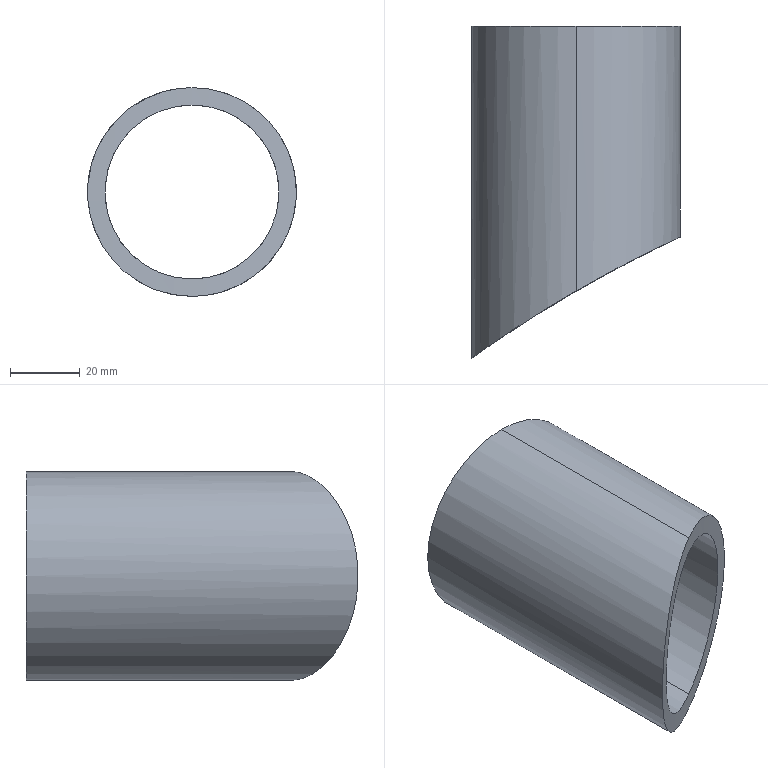Part | SolidWorks | features Extrusion 1, ICE 1 | 1 solid | 6 faces | box 60 x 95.435 x 60 mm | volume 66487 mm3 | cylinder 5 | plane 1 | commonest cylinder face diameters 50 x2 60 x2 759 x1
STEP:
#1=CARTESIAN_POINT('',(0.,300.,-25.));
#2=VERTEX_POINT('',#1);
#3=CARTESIAN_POINT('',(0.,300.,25.));
#4=VERTEX_POINT('',#3);
#5=CARTESIAN_POINT('',(0.,300.,0.));
#6=DIRECTION('',(0.,1.,0.));
#7=DIRECTION('',(0.,0.,1.));
#8=AXIS2_PLACEMENT_3D('',#5,#6,#7);
#9=CIRCLE('',#8,25.);
#10=EDGE_CURVE('',#2,#4,#9,.T.);
#11=ORIENTED_EDGE('',*,*,#10,.T.);
#12=CARTESIAN_POINT('',(0.,223.819,25.));
#13=VERTEX_POINT('',#12);
#14=CARTESIAN_POINT('',(0.,300.,25.));
#15=DIRECTION('',(0.,-1.,0.));
#16=VECTOR('',#15,1000.);
#17=LINE('',#14,#16);
#18=EDGE_CURVE('',#4,#13,#17,.T.);
#19=ORIENTED_EDGE('',*,*,#18,.T.);
#20=CARTESIAN_POINT('',(0.,223.819,-25.));
#21=VERTEX_POINT('',#20);
#22=CARTESIAN_POINT('',(0.,223.819,-25.));
#23=CARTESIAN_POINT('',(-1.557,222.92,-25.));
#24=CARTESIAN_POINT('',(-3.084,222.023,-24.856));
#25=CARTESIAN_POINT('',(-6.08,220.237,-24.297));
#26=CARTESIAN_POINT('',(-7.55,219.347,-23.883));
#27=CARTESIAN_POINT('',(-9.35,218.24,-23.189));
#28=CARTESIAN_POINT('',(-9.708,218.019,-23.041));
#29=CARTESIAN_POINT('',(-10.421,217.578,-22.728));
#30=CARTESIAN_POINT('',(-10.777,217.357,-22.561));
#31=CARTESIAN_POINT('',(-11.828,216.701,-22.039));
#32=CARTESIAN_POINT('',(-12.511,216.272,-21.658));
#33=CARTESIAN_POINT('',(-14.504,215.01,-20.422));
#34=CARTESIAN_POINT('',(-15.76,214.204,-19.473));
#35=CARTESIAN_POINT('',(-17.529,213.055,-17.843));
#36=CARTESIAN_POINT('',(-18.1,212.683,-17.265));
#37=CARTESIAN_POINT('',(-19.198,211.96,-16.034));
#38=CARTESIAN_POINT('',(-19.719,211.617,-15.39));
#39=CARTESIAN_POINT('',(-21.185,210.643,-13.377));
#40=CARTESIAN_POINT('',(-22.041,210.068,-11.926));
#41=CARTESIAN_POINT('',(-22.937,209.462,-9.953));
#42=CARTESIAN_POINT('',(-23.108,209.346,-9.551));
#43=CARTESIAN_POINT('',(-23.426,209.131,-8.741));
#44=CARTESIAN_POINT('',(-23.575,209.03,-8.333));
#45=CARTESIAN_POINT('',(-23.988,208.749,-7.095));
#46=CARTESIAN_POINT('',(-24.221,208.59,-6.254));
#47=CARTESIAN_POINT('',(-24.6,208.331,-4.541));
#48=CARTESIAN_POINT('',(-24.746,208.231,-3.669));
#49=CARTESIAN_POINT('',(-24.895,208.128,-2.334));
#50=CARTESIAN_POINT('',(-24.933,208.102,-1.883));
#51=CARTESIAN_POINT('',(-24.985,208.067,-0.9858));
#52=CARTESIAN_POINT('',(-24.998,208.057,-0.5381));
#53=CARTESIAN_POINT('',(-25.006,208.052,1.694));
#54=CARTESIAN_POINT('',(-24.824,208.177,3.462));
#55=CARTESIAN_POINT('',(-24.078,208.687,6.959));
#56=CARTESIAN_POINT('',(-23.531,209.061,8.619));
#57=CARTESIAN_POINT('',(-22.651,209.656,10.589));
#58=CARTESIAN_POINT('',(-22.465,209.781,10.978));
#59=CARTESIAN_POINT('',(-22.073,210.045,11.745));
#60=CARTESIAN_POINT('',(-21.868,210.183,12.123));
#61=CARTESIAN_POINT('',(-21.23,210.611,13.229));
#62=CARTESIAN_POINT('',(-20.773,210.916,13.935));
#63=CARTESIAN_POINT('',(-19.8,211.562,15.285));
#64=CARTESIAN_POINT('',(-19.285,211.904,15.93));
#65=CARTESIAN_POINT('',(-18.196,212.62,17.164));
#66=CARTESIAN_POINT('',(-17.621,212.995,17.753));
#67=CARTESIAN_POINT('',(-15.844,214.15,19.406));
#68=CARTESIAN_POINT('',(-14.581,214.962,20.369));
#69=CARTESIAN_POINT('',(-12.909,216.02,21.413));
#70=CARTESIAN_POINT('',(-12.57,216.234,21.614));
#71=CARTESIAN_POINT('',(-11.883,216.666,21.999));
#72=CARTESIAN_POINT('',(-11.534,216.884,22.184));
#73=CARTESIAN_POINT('',(-10.482,217.541,22.71));
#74=CARTESIAN_POINT('',(-9.771,217.981,23.024));
#75=CARTESIAN_POINT('',(-7.609,219.311,23.864));
#76=CARTESIAN_POINT('',(-6.129,220.208,24.286));
#77=CARTESIAN_POINT('',(-3.851,221.566,24.714));
#78=CARTESIAN_POINT('',(-3.079,222.023,24.822));
#79=CARTESIAN_POINT('',(-1.539,222.926,24.965));
#80=CARTESIAN_POINT('',(-0.7698,223.374,25.));
#81=CARTESIAN_POINT('',(0.,223.819,25.));
#82=B_SPLINE_CURVE_WITH_KNOTS('',3,(#22,#23,#24,#25,#26,#27,#28,#29,#30,#31,#32,#33,#34,#35,#36,#37,#38,#39,#40,#41,#42,#43,#44,#45,#46,#47,#48,#49,#50,#51,#52,#53,#54,#55,#56,#57,#58,#59,#60,#61,#62,#63,#64,#65,#66,#67,#68,#69,#70,#71,#72,#73,#74,#75,#76,#77,#78,#79,#80,#81),.UNSPECIFIED.,.F.,.F.,(4,2,2,2,2,2,2,2,2,2,2,2,2,2,2,2,2,2,2,2,2,2,2,2,2,2,2,2,2,4),(0.,0.005296,0.01059,0.01192,0.01324,0.01589,0.02118,0.02383,0.02648,0.03178,0.0331,0.03442,0.03707,0.03972,0.04104,0.04237,0.04766,0.05296,0.05429,0.05561,0.05826,0.06091,0.06355,0.06885,0.07017,0.0715,0.07415,0.07944,0.08209,0.08474),.UNSPECIFIED.);
#83=EDGE_CURVE('',#21,#13,#82,.T.);
#84=ORIENTED_EDGE('',*,*,#83,.F.);
#85=CARTESIAN_POINT('',(0.,300.,-25.));
#86=DIRECTION('',(0.,-1.,0.));
#87=VECTOR('',#86,1000.);
#88=LINE('',#85,#87);
#89=EDGE_CURVE('',#2,#21,#88,.T.);
#90=ORIENTED_EDGE('',*,*,#89,.F.);
#91=EDGE_LOOP('',(#11,#19,#84,#90));
#92=FACE_OUTER_BOUND('',#91,.T.);
#93=CARTESIAN_POINT('',(0.,300.,0.));
#94=DIRECTION('',(0.,-1.,0.));
#95=DIRECTION('',(0.,0.,-1.));
#96=AXIS2_PLACEMENT_3D('',#93,#94,#95);
#97=CYLINDRICAL_SURFACE('',#96,25.);
#98=ADVANCED_FACE('',(#92),#97,.F.);
#99=CARTESIAN_POINT('',(0.,300.,30.));
#100=VERTEX_POINT('',#99);
#101=CARTESIAN_POINT('',(0.,300.,-30.));
#102=VERTEX_POINT('',#101);
#103=CARTESIAN_POINT('',(0.,300.,0.));
#104=DIRECTION('',(0.,1.,0.));
#105=DIRECTION('',(0.,0.,1.));
#106=AXIS2_PLACEMENT_3D('',#103,#104,#105);
#107=CIRCLE('',#106,30.);
#108=EDGE_CURVE('',#100,#102,#107,.T.);
#109=ORIENTED_EDGE('',*,*,#108,.F.);
#110=CARTESIAN_POINT('',(0.,223.819,30.));
#111=VERTEX_POINT('',#110);
#112=CARTESIAN_POINT('',(0.,300.,30.));
#113=DIRECTION('',(0.,-1.,0.));
#114=VECTOR('',#113,1000.);
#115=LINE('',#112,#114);
#116=EDGE_CURVE('',#100,#111,#115,.T.);
#117=ORIENTED_EDGE('',*,*,#116,.T.);
#118=CARTESIAN_POINT('',(0.,223.819,-30.));
#119=VERTEX_POINT('',#118);
#120=CARTESIAN_POINT('',(0.,223.819,30.));
#121=CARTESIAN_POINT('',(1.801,224.858,30.));
#122=CARTESIAN_POINT('',(3.604,225.88,29.839));
#123=CARTESIAN_POINT('',(5.861,227.134,29.425));
#124=CARTESIAN_POINT('',(6.313,227.384,29.332));
#125=CARTESIAN_POINT('',(7.216,227.881,29.123));
#126=CARTESIAN_POINT('',(7.668,228.128,29.007));
#127=CARTESIAN_POINT('',(9.01,228.86,28.63));
#128=CARTESIAN_POINT('',(9.892,229.336,28.338));
#129=CARTESIAN_POINT('',(12.496,230.729,27.337));
#130=CARTESIAN_POINT('',(14.179,231.612,26.506));
#131=CARTESIAN_POINT('',(16.614,232.868,24.998));
#132=CARTESIAN_POINT('',(17.412,233.275,24.449));
#133=CARTESIAN_POINT('',(18.969,234.064,23.263));
#134=CARTESIAN_POINT('',(19.716,234.44,22.633));
#135=CARTESIAN_POINT('',(21.865,235.511,20.634));
#136=CARTESIAN_POINT('',(23.174,236.152,19.157));
#137=CARTESIAN_POINT('',(24.642,236.863,17.118));
#138=CARTESIAN_POINT('',(24.927,237.001,16.7));
#139=CARTESIAN_POINT('',(25.479,237.267,15.845));
#140=CARTESIAN_POINT('',(25.747,237.395,15.406));
#141=CARTESIAN_POINT('',(26.514,237.762,14.074));
#142=CARTESIAN_POINT('',(26.978,237.982,13.163));
#143=CARTESIAN_POINT('',(28.228,238.574,10.362));
#144=CARTESIAN_POINT('',(28.875,238.877,8.404));
#145=CARTESIAN_POINT('',(29.432,239.136,5.836));
#146=CARTESIAN_POINT('',(29.53,239.182,5.317));
#147=CARTESIAN_POINT('',(29.697,239.26,4.282));
#148=CARTESIAN_POINT('',(29.768,239.293,3.764));
#149=CARTESIAN_POINT('',(29.937,239.371,2.207));
#150=CARTESIAN_POINT('',(29.995,239.399,1.166));
#151=CARTESIAN_POINT('',(30.004,239.403,-0.9206));
#152=CARTESIAN_POINT('',(29.954,239.379,-1.967));
#153=CARTESIAN_POINT('',(29.795,239.305,-3.541));
#154=CARTESIAN_POINT('',(29.728,239.274,-4.066));
#155=CARTESIAN_POINT('',(29.567,239.2,-5.103));
#156=CARTESIAN_POINT('',(29.474,239.156,-5.617));
#157=CARTESIAN_POINT('',(28.942,238.908,-8.167));
#158=CARTESIAN_POINT('',(28.311,238.613,-10.138));
#159=CARTESIAN_POINT('',(27.269,238.12,-12.516));
#160=CARTESIAN_POINT('',(27.049,238.016,-12.985));
#161=CARTESIAN_POINT('',(26.588,237.797,-13.905));
#162=CARTESIAN_POINT('',(26.347,237.682,-14.356));
#163=CARTESIAN_POINT('',(25.593,237.322,-15.685));
#164=CARTESIAN_POINT('',(25.05,237.06,-16.539));
#165=CARTESIAN_POINT('',(23.884,236.496,-18.181));
#166=CARTESIAN_POINT('',(23.262,236.194,-18.971));
#167=CARTESIAN_POINT('',(21.939,235.545,-20.487));
#168=CARTESIAN_POINT('',(21.247,235.203,-21.202));
#169=CARTESIAN_POINT('',(19.095,234.13,-23.222));
#170=CARTESIAN_POINT('',(17.555,233.352,-24.404));
#171=CARTESIAN_POINT('',(15.508,232.297,-25.685));
#172=CARTESIAN_POINT('',(15.092,232.082,-25.932));
#173=CARTESIAN_POINT('',(14.256,231.647,-26.401));
#174=CARTESIAN_POINT('',(13.835,231.427,-26.624));
#175=CARTESIAN_POINT('',(12.562,230.759,-27.26));
#176=CARTESIAN_POINT('',(11.702,230.304,-27.64));
#177=CARTESIAN_POINT('',(9.958,229.372,-28.314));
#178=CARTESIAN_POINT('',(9.075,228.895,-28.609));
#179=CARTESIAN_POINT('',(7.288,227.922,-29.116));
#180=CARTESIAN_POINT('',(6.38,227.422,-29.328));
#181=CARTESIAN_POINT('',(4.562,226.412,-29.666));
#182=CARTESIAN_POINT('',(3.651,225.902,-29.791));
#183=CARTESIAN_POINT('',(2.283,225.127,-29.916));
#184=CARTESIAN_POINT('',(1.827,224.867,-29.948));
#185=CARTESIAN_POINT('',(0.9141,224.345,-29.99));
#186=CARTESIAN_POINT('',(0.4556,224.082,-30.));
#187=CARTESIAN_POINT('',(0.,223.819,-30.));
#188=B_SPLINE_CURVE_WITH_KNOTS('',3,(#120,#121,#122,#123,#124,#125,#126,#127,#128,#129,#130,#131,#132,#133,#134,#135,#136,#137,#138,#139,#140,#141,#142,#143,#144,#145,#146,#147,#148,#149,#150,#151,#152,#153,#154,#155,#156,#157,#158,#159,#160,#161,#162,#163,#164,#165,#166,#167,#168,#169,#170,#171,#172,#173,#174,#175,#176,#177,#178,#179,#180,#181,#182,#183,#184,#185,#186,#187),.UNSPECIFIED.,.F.,.F.,(4,2,2,2,2,2,2,2,2,2,2,2,2,2,2,2,2,2,2,2,2,2,2,2,2,2,2,2,2,2,2,2,2,4),(0.102,0.1082,0.1097,0.1113,0.1144,0.1206,0.1236,0.1267,0.1329,0.1345,0.136,0.1391,0.1453,0.1469,0.1484,0.1515,0.1546,0.1562,0.1577,0.1639,0.1655,0.167,0.1701,0.1732,0.1763,0.1825,0.1841,0.1856,0.1887,0.1918,0.1949,0.198,0.1996,0.2011),.UNSPECIFIED.);
#189=EDGE_CURVE('',#111,#119,#188,.T.);
#190=ORIENTED_EDGE('',*,*,#189,.T.);
#191=CARTESIAN_POINT('',(0.,300.,-30.));
#192=DIRECTION('',(0.,-1.,0.));
#193=VECTOR('',#192,1000.);
#194=LINE('',#191,#193);
#195=EDGE_CURVE('',#102,#119,#194,.T.);
#196=ORIENTED_EDGE('',*,*,#195,.F.);
#197=EDGE_LOOP('',(#109,#117,#190,#196));
#198=FACE_OUTER_BOUND('',#197,.T.);
#199=CARTESIAN_POINT('',(0.,300.,0.));
#200=DIRECTION('',(0.,-1.,0.));
#201=DIRECTION('',(0.,0.,-1.));
#202=AXIS2_PLACEMENT_3D('',#199,#200,#201);
#203=CYLINDRICAL_SURFACE('',#202,30.);
#204=ADVANCED_FACE('',(#198),#203,.T.);
#205=CARTESIAN_POINT('',(0.,300.,0.));
#206=DIRECTION('',(0.,1.,0.));
#207=DIRECTION('',(0.,0.,1.));
#208=AXIS2_PLACEMENT_3D('',#205,#206,#207);
#209=CIRCLE('',#208,30.);
#210=EDGE_CURVE('',#102,#100,#209,.T.);
#211=ORIENTED_EDGE('',*,*,#210,.T.);
#212=ORIENTED_EDGE('',*,*,#108,.T.);
#213=EDGE_LOOP('',(#211,#212));
#214=FACE_OUTER_BOUND('',#213,.T.);
#215=ORIENTED_EDGE('',*,*,#10,.F.);
#216=CARTESIAN_POINT('',(0.,300.,0.));
#217=DIRECTION('',(0.,1.,0.));
#218=DIRECTION('',(0.,0.,1.));
#219=AXIS2_PLACEMENT_3D('',#216,#217,#218);
#220=CIRCLE('',#219,25.);
#221=EDGE_CURVE('',#4,#2,#220,.T.);
#222=ORIENTED_EDGE('',*,*,#221,.F.);
#223=EDGE_LOOP('',(#215,#222));
#224=FACE_BOUND('',#223,.T.);
#225=CARTESIAN_POINT('',(0.,300.,0.));
#226=DIRECTION('',(0.,1.,0.));
#227=DIRECTION('',(0.,0.,1.));
#228=AXIS2_PLACEMENT_3D('',#225,#226,#227);
#229=PLANE('',#228);
#230=ADVANCED_FACE('',(#214,#224),#229,.T.);
#231=ORIENTED_EDGE('',*,*,#116,.F.);
#232=ORIENTED_EDGE('',*,*,#210,.F.);
#233=ORIENTED_EDGE('',*,*,#195,.T.);
#234=CARTESIAN_POINT('',(0.,223.819,-30.));
#235=CARTESIAN_POINT('',(-1.874,222.737,-30.));
#236=CARTESIAN_POINT('',(-3.709,221.656,-29.826));
#237=CARTESIAN_POINT('',(-7.307,219.497,-29.154));
#238=CARTESIAN_POINT('',(-9.071,218.418,-28.656));
#239=CARTESIAN_POINT('',(-11.23,217.074,-27.823));
#240=CARTESIAN_POINT('',(-11.66,216.806,-27.645));
#241=CARTESIAN_POINT('',(-12.515,216.269,-27.269));
#242=CARTESIAN_POINT('',(-12.941,216.,-27.07));
#243=CARTESIAN_POINT('',(-14.201,215.202,-26.443));
#244=CARTESIAN_POINT('',(-15.019,214.679,-25.987));
#245=CARTESIAN_POINT('',(-17.406,213.14,-24.506));
#246=CARTESIAN_POINT('',(-18.911,212.154,-23.368));
#247=CARTESIAN_POINT('',(-21.03,210.745,-21.416));
#248=CARTESIAN_POINT('',(-21.714,210.288,-20.724));
#249=CARTESIAN_POINT('',(-23.03,209.4,-19.25));
#250=CARTESIAN_POINT('',(-23.654,208.977,-18.479));
#251=CARTESIAN_POINT('',(-25.412,207.776,-16.068));
#252=CARTESIAN_POINT('',(-26.439,207.065,-14.328));
#253=CARTESIAN_POINT('',(-27.517,206.314,-11.961));
#254=CARTESIAN_POINT('',(-27.722,206.17,-11.479));
#255=CARTESIAN_POINT('',(-28.105,205.903,-10.507));
#256=CARTESIAN_POINT('',(-28.283,205.777,-10.017));
#257=CARTESIAN_POINT('',(-28.78,205.428,-8.531));
#258=CARTESIAN_POINT('',(-29.061,205.23,-7.522));
#259=CARTESIAN_POINT('',(-29.517,204.907,-5.463));
#260=CARTESIAN_POINT('',(-29.693,204.783,-4.414));
#261=CARTESIAN_POINT('',(-29.873,204.655,-2.809));
#262=CARTESIAN_POINT('',(-29.919,204.622,-2.267));
#263=CARTESIAN_POINT('',(-29.981,204.578,-1.187));
#264=CARTESIAN_POINT('',(-29.998,204.567,-0.6484));
#265=CARTESIAN_POINT('',(-30.008,204.56,2.037));
#266=CARTESIAN_POINT('',(-29.787,204.716,4.163));
#267=CARTESIAN_POINT('',(-28.889,205.352,8.37));
#268=CARTESIAN_POINT('',(-28.23,205.816,10.361));
#269=CARTESIAN_POINT('',(-26.96,206.702,13.199));
#270=CARTESIAN_POINT('',(-26.487,207.031,14.125));
#271=CARTESIAN_POINT('',(-25.466,207.737,15.892));
#272=CARTESIAN_POINT('',(-24.918,208.113,16.736));
#273=CARTESIAN_POINT('',(-23.751,208.911,18.355));
#274=CARTESIAN_POINT('',(-23.132,209.331,19.128));
#275=CARTESIAN_POINT('',(-22.152,209.992,20.236));
#276=CARTESIAN_POINT('',(-21.816,210.218,20.598));
#277=CARTESIAN_POINT('',(-21.132,210.677,21.3));
#278=CARTESIAN_POINT('',(-20.783,210.909,21.64));
#279=CARTESIAN_POINT('',(-19.01,212.088,23.289));
#280=CARTESIAN_POINT('',(-17.497,213.081,24.442));
#281=CARTESIAN_POINT('',(-15.092,214.632,25.945));
#282=CARTESIAN_POINT('',(-14.264,215.161,26.409));
#283=CARTESIAN_POINT('',(-12.585,216.225,27.249));
#284=CARTESIAN_POINT('',(-11.733,216.761,27.626));
#285=CARTESIAN_POINT('',(-9.142,218.375,28.633));
#286=CARTESIAN_POINT('',(-7.366,219.462,29.141));
#287=CARTESIAN_POINT('',(-4.627,221.105,29.656));
#288=CARTESIAN_POINT('',(-3.699,221.657,29.785));
#289=CARTESIAN_POINT('',(-1.851,222.745,29.957));
#290=CARTESIAN_POINT('',(-0.9257,223.284,30.));
#291=CARTESIAN_POINT('',(0.,223.819,30.));
#292=B_SPLINE_CURVE_WITH_KNOTS('',3,(#234,#235,#236,#237,#238,#239,#240,#241,#242,#243,#244,#245,#246,#247,#248,#249,#250,#251,#252,#253,#254,#255,#256,#257,#258,#259,#260,#261,#262,#263,#264,#265,#266,#267,#268,#269,#270,#271,#272,#273,#274,#275,#276,#277,#278,#279,#280,#281,#282,#283,#284,#285,#286,#287,#288,#289,#290,#291),.UNSPECIFIED.,.F.,.F.,(4,2,2,2,2,2,2,2,2,2,2,2,2,2,2,2,2,2,2,2,2,2,2,2,2,2,2,2,4),(0.,0.006372,0.01274,0.01434,0.01593,0.01912,0.02549,0.02867,0.03186,0.03823,0.03983,0.04142,0.04461,0.04779,0.04938,0.05098,0.05735,0.06372,0.06691,0.07009,0.07328,0.07487,0.07647,0.08284,0.08602,0.08921,0.09558,0.09877,0.102),.UNSPECIFIED.);
#293=EDGE_CURVE('',#119,#111,#292,.T.);
#294=ORIENTED_EDGE('',*,*,#293,.T.);
#295=EDGE_LOOP('',(#231,#232,#233,#294));
#296=FACE_OUTER_BOUND('',#295,.T.);
#297=CARTESIAN_POINT('',(0.,300.,0.));
#298=DIRECTION('',(0.,-1.,0.));
#299=DIRECTION('',(0.,0.,-1.));
#300=AXIS2_PLACEMENT_3D('',#297,#298,#299);
#301=CYLINDRICAL_SURFACE('',#300,30.);
#302=ADVANCED_FACE('',(#296),#301,.T.);
#303=ORIENTED_EDGE('',*,*,#18,.F.);
#304=ORIENTED_EDGE('',*,*,#221,.T.);
#305=ORIENTED_EDGE('',*,*,#89,.T.);
#306=CARTESIAN_POINT('',(0.,223.819,25.));
#307=CARTESIAN_POINT('',(1.504,224.687,25.));
#308=CARTESIAN_POINT('',(3.008,225.542,24.865));
#309=CARTESIAN_POINT('',(4.889,226.593,24.52));
#310=CARTESIAN_POINT('',(5.265,226.803,24.442));
#311=CARTESIAN_POINT('',(6.017,227.22,24.268));
#312=CARTESIAN_POINT('',(6.394,227.428,24.172));
#313=CARTESIAN_POINT('',(7.513,228.044,23.857));
#314=CARTESIAN_POINT('',(8.247,228.445,23.613));
#315=CARTESIAN_POINT('',(10.417,229.621,22.779));
#316=CARTESIAN_POINT('',(11.818,230.367,22.088));
#317=CARTESIAN_POINT('',(13.843,231.432,20.833));
#318=CARTESIAN_POINT('',(14.505,231.778,20.378));
#319=CARTESIAN_POINT('',(15.802,232.45,19.39));
#320=CARTESIAN_POINT('',(16.425,232.77,18.865));
#321=CARTESIAN_POINT('',(18.214,233.685,17.202));
#322=CARTESIAN_POINT('',(19.304,234.234,15.973));
#323=CARTESIAN_POINT('',(20.527,234.844,14.277));
#324=CARTESIAN_POINT('',(20.764,234.962,13.93));
#325=CARTESIAN_POINT('',(21.224,235.19,13.218));
#326=CARTESIAN_POINT('',(21.447,235.301,12.853));
#327=CARTESIAN_POINT('',(22.087,235.617,11.742));
#328=CARTESIAN_POINT('',(22.475,235.808,10.982));
#329=CARTESIAN_POINT('',(23.519,236.319,8.647));
#330=CARTESIAN_POINT('',(24.059,236.581,7.016));
#331=CARTESIAN_POINT('',(24.524,236.806,4.876));
#332=CARTESIAN_POINT('',(24.606,236.846,4.442));
#333=CARTESIAN_POINT('',(24.747,236.914,3.578));
#334=CARTESIAN_POINT('',(24.805,236.942,3.145));
#335=CARTESIAN_POINT('',(24.947,237.01,1.844));
#336=CARTESIAN_POINT('',(24.996,237.034,0.9753));
#337=CARTESIAN_POINT('',(25.003,237.038,-0.7665));
#338=CARTESIAN_POINT('',(24.962,237.017,-1.639));
#339=CARTESIAN_POINT('',(24.829,236.953,-2.952));
#340=CARTESIAN_POINT('',(24.773,236.926,-3.39));
#341=CARTESIAN_POINT('',(24.639,236.862,-4.257));
#342=CARTESIAN_POINT('',(24.561,236.824,-4.687));
#343=CARTESIAN_POINT('',(24.116,236.609,-6.816));
#344=CARTESIAN_POINT('',(23.589,236.353,-8.459));
#345=CARTESIAN_POINT('',(22.72,235.928,-10.44));
#346=CARTESIAN_POINT('',(22.536,235.837,-10.832));
#347=CARTESIAN_POINT('',(22.151,235.648,-11.598));
#348=CARTESIAN_POINT('',(21.95,235.549,-11.975));
#349=CARTESIAN_POINT('',(21.321,235.239,-13.082));
#350=CARTESIAN_POINT('',(20.868,235.014,-13.793));
#351=CARTESIAN_POINT('',(19.896,234.529,-15.161));
#352=CARTESIAN_POINT('',(19.377,234.269,-15.818));
#353=CARTESIAN_POINT('',(18.276,233.714,-17.079));
#354=CARTESIAN_POINT('',(17.699,233.421,-17.675));
#355=CARTESIAN_POINT('',(15.907,232.506,-19.356));
#356=CARTESIAN_POINT('',(14.626,231.843,-20.339));
#357=CARTESIAN_POINT('',(12.923,230.948,-21.405));
#358=CARTESIAN_POINT('',(12.576,230.766,-21.61));
#359=CARTESIAN_POINT('',(11.88,230.397,-22.));
#360=CARTESIAN_POINT('',(11.53,230.211,-22.186));
#361=CARTESIAN_POINT('',(10.47,229.646,-22.716));
#362=CARTESIAN_POINT('',(9.754,229.261,-23.032));
#363=CARTESIAN_POINT('',(8.302,228.475,-23.594));
#364=CARTESIAN_POINT('',(7.567,228.074,-23.84));
#365=CARTESIAN_POINT('',(6.079,227.255,-24.262));
#366=CARTESIAN_POINT('',(5.323,226.836,-24.439));
#367=CARTESIAN_POINT('',(3.806,225.988,-24.721));
#368=CARTESIAN_POINT('',(3.047,225.56,-24.825));
#369=CARTESIAN_POINT('',(1.906,224.912,-24.93));
#370=CARTESIAN_POINT('',(1.525,224.695,-24.956));
#371=CARTESIAN_POINT('',(0.763,224.258,-24.991));
#372=CARTESIAN_POINT('',(0.3804,224.038,-25.));
#373=CARTESIAN_POINT('',(0.,223.819,-25.));
#374=B_SPLINE_CURVE_WITH_KNOTS('',3,(#306,#307,#308,#309,#310,#311,#312,#313,#314,#315,#316,#317,#318,#319,#320,#321,#322,#323,#324,#325,#326,#327,#328,#329,#330,#331,#332,#333,#334,#335,#336,#337,#338,#339,#340,#341,#342,#343,#344,#345,#346,#347,#348,#349,#350,#351,#352,#353,#354,#355,#356,#357,#358,#359,#360,#361,#362,#363,#364,#365,#366,#367,#368,#369,#370,#371,#372,#373),.UNSPECIFIED.,.F.,.F.,(4,2,2,2,2,2,2,2,2,2,2,2,2,2,2,2,2,2,2,2,2,2,2,2,2,2,2,2,2,2,2,2,2,4),(0.08474,0.08991,0.09121,0.0925,0.09509,0.1003,0.1028,0.1054,0.1106,0.1119,0.1132,0.1158,0.121,0.1223,0.1235,0.1261,0.1287,0.13,0.1313,0.1365,0.1378,0.1391,0.1417,0.1442,0.1468,0.152,0.1533,0.1546,0.1572,0.1598,0.1624,0.1649,0.1662,0.1675),.UNSPECIFIED.);
#375=EDGE_CURVE('',#13,#21,#374,.T.);
#376=ORIENTED_EDGE('',*,*,#375,.F.);
#377=EDGE_LOOP('',(#303,#304,#305,#376));
#378=FACE_OUTER_BOUND('',#377,.T.);
#379=CARTESIAN_POINT('',(0.,300.,0.));
#380=DIRECTION('',(0.,-1.,0.));
#381=DIRECTION('',(0.,0.,-1.));
#382=AXIS2_PLACEMENT_3D('',#379,#380,#381);
#383=CYLINDRICAL_SURFACE('',#382,25.);
#384=ADVANCED_FACE('',(#378),#383,.F.);
#385=ORIENTED_EDGE('',*,*,#83,.T.);
#386=ORIENTED_EDGE('',*,*,#375,.T.);
#387=EDGE_LOOP('',(#385,#386));
#388=FACE_BOUND('',#387,.T.);
#389=ORIENTED_EDGE('',*,*,#293,.F.);
#390=ORIENTED_EDGE('',*,*,#189,.F.);
#391=EDGE_LOOP('',(#389,#390));
#392=FACE_OUTER_BOUND('',#391,.T.);
#393=CARTESIAN_POINT('',(189.75,-104.838,-30.));
#394=DIRECTION('',(0.,0.,1.));
#395=DIRECTION('',(1.,0.,0.));
#396=AXIS2_PLACEMENT_3D('',#393,#394,#395);
#397=CYLINDRICAL_SURFACE('',#396,379.5);
#398=ADVANCED_FACE('',(#388,#392),#397,.F.);
#399=CLOSED_SHELL('',(#98,#204,#230,#302,#384,#398));
#400=MANIFOLD_SOLID_BREP('',#399);
#401=CARTESIAN_POINT('',(0.,0.,0.));
#402=DIRECTION('',(0.,0.,1.));
#403=DIRECTION('',(1.,0.,0.));
#404=AXIS2_PLACEMENT_3D('',#401,#402,#403);
#405=(LENGTH_UNIT()NAMED_UNIT(*)SI_UNIT(.MILLI.,.METRE.));
#406=UNCERTAINTY_MEASURE_WITH_UNIT(LENGTH_MEASURE(0.00001),#405,'','');
#407=(NAMED_UNIT(*)PLANE_ANGLE_UNIT()SI_UNIT($,.RADIAN.));
#408=(NAMED_UNIT(*)SI_UNIT($,.STERADIAN.)SOLID_ANGLE_UNIT());
#409=(GEOMETRIC_REPRESENTATION_CONTEXT(3)GLOBAL_UNCERTAINTY_ASSIGNED_CONTEXT((#406))GLOBAL_UNIT_ASSIGNED_CONTEXT((#405,#407,#408))REPRESENTATION_CONTEXT('',''));
#410=ADVANCED_BREP_SHAPE_REPRESENTATION('',(#400,#404),#409);